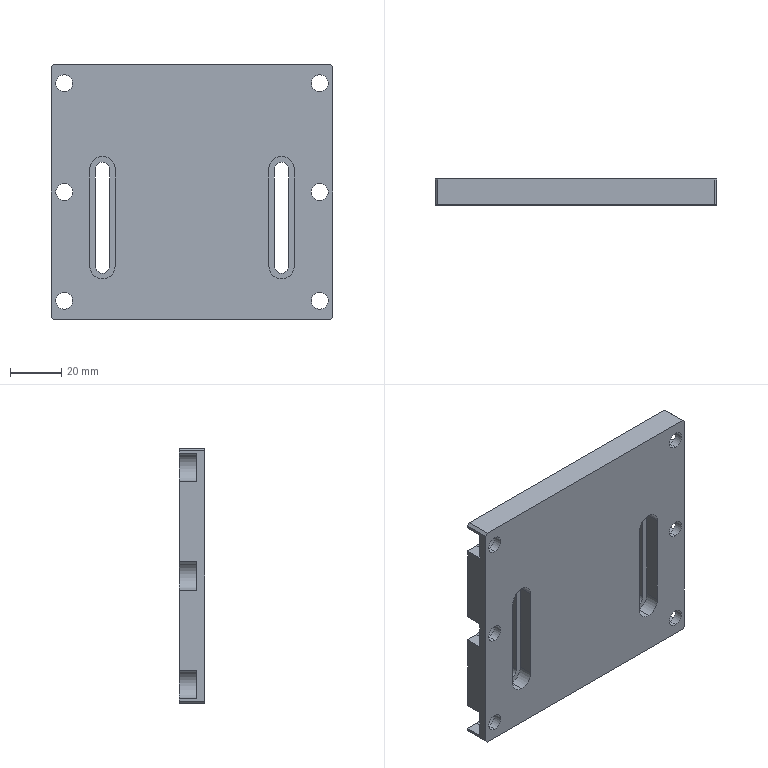Part | STEP file | 0-19-15 Cylinder connecting plate | 1 solid | 68 faces | box 110 x 10 x 100 mm | volume 97973 mm3 | plane 38 | cylinder 30 | commonest cylinder face diameters 6.6 x12 5.5 x6 9.9 x6 11 x6